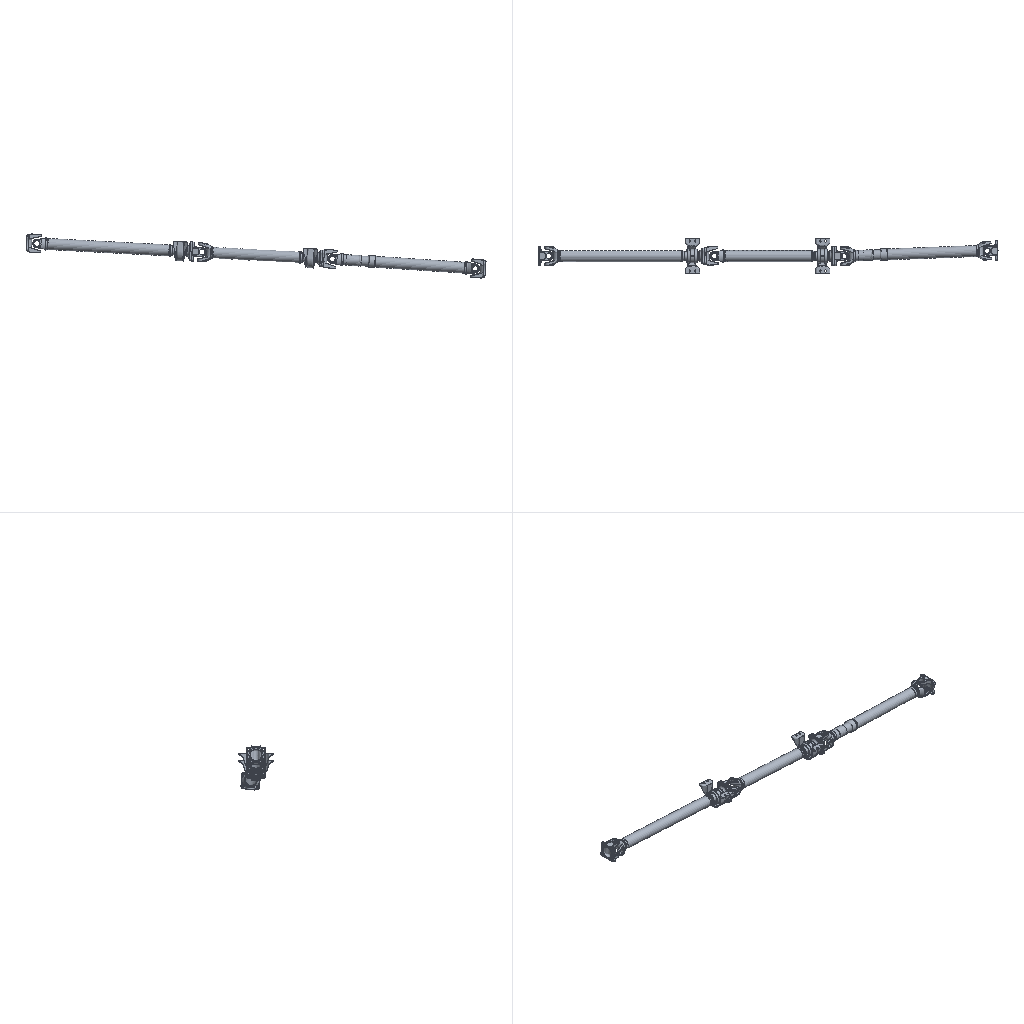Simulation study | nastran
Set-up summary:
category,name,step,type,value,unit,region
solver,nx_nastran
units,not stated in the deck,,not stated
analysis,deck,,modal,modal
analysis,solution,,SOL,103
load_step,SUBCASE 1,1,SUBCASE,SPC=1 LOAD=None
mesh,nodes,,,200329
mesh,elements,,,777144
element_type,CQUAD4,,shell,9182
element_type,CTETRA,,solid,767674
element_type,CTRIA3,,shell,288
load,load commands in deck,,count,0
bc,support commands in deck,,count,16
check,setup vs results,,match,"every grid point's frame and coordinates and every element id; grid points of CQUAD4, CTETRA, CTRIA3 elements"
Nastran input file, long lists of numbers shortened:
$$------------------------------------------------------------------------------$
$$                                                                              $
$$ NASTRAN Input Deck Generated by HyperMesh Version  :10.0buil                 $
$$ Generated using HyperMesh-Nastran Template Version : 10.0build60
$$                                                                              $
$$   Template:  general                                                         $
$$                                                                              $
$$------------------------------------------------------------------------------$
$$------------------------------------------------------------------------------$
$$                      Executive Control Cards                                 $
$$------------------------------------------------------------------------------$
SOL 103
CEND
$$------------------------------------------------------------------------------$
$$                      Case Control Cards                                      $
$$------------------------------------------------------------------------------$
  DISPLACEMENT = ALL
$
$HMNAME LOADSTEP               1"modal"
SUBCASE       1
  LABEL=  modal
  SPC =        1
  METHOD(STRUCTURE) =        2
$$------------------------------------------------------------------------------$
$$                      Bulk Data Cards                                         $
$$------------------------------------------------------------------------------$
BEGIN BULK
PARAM,POST,-1
$$
$$  GRID Data
$$
GRID           1        4926.96494.71653-393.548
GRID           2        4929.61194.74233-394.182
$ (200327 more lines like these left out)
$$
$$  SPOINT Data
$$
$$
$$------------------------------------------------------------------------------$
$$             Group Definitions                                                $
$$------------------------------------------------------------------------------$
$
$ RBE2 Elements - Single dependent node
$
RBE2      149214   28273   12346   28272
RBE2      618930  160318   12346  160317
$
$HMMOVE       10
$         149214  618930
$
$$
$$ RBE2 Elements - Multiple dependent nodes
$$
RBE2      149212   28272   12345    3911    3912    3913    3914    3915+
+           3916    3917    3918    3919    3920    3921    3922    4886+
+           4887    4888    4889    4890    4891    4892    4893    4894+
+           4895    4896    4897    4898    4899    4900    4901    4902+
+           4903    4904    4905    4906    4907    4908    4909    4910+
+           4911    4912    4913    4914    4915    4916    4917    4918+
+           4919    4920    4921    4922    4923    4924    4925    4926+
+           4927    4928    4929    4930    4931    4932    4933    4934+
+           5993    5994    5995    5996    5997    5998    5999    6000+
+           6001    6002    6003    6004    6005    6006    6007    6008+
+           6009    6010    6011    6012    6013    6014    6015    6016+
+           6017    6018    6179    6180    6181    6182    6183    6184+
+           6185    6186    6187    6188    6189    6190    6191    6192+
+           6193    6194    6195    6196    6197    6198    6199    6200+
+           6201    6202    6203    6204    6205    6206    6207    6208+
+           6209    6210    6211    6212    6213    6214    6215    6216+
+           6217    6218    6219    6220    6221    6222    6223    6224+
+           6225    6226    6227    6228    6229    6230    6231    6232+
+           6233    6234    6235    6236    6237    6238    6239    6240+
+           6241    6242    6243    6244    6245    6246    6247    6248+
+           6249    6250    6251    6252    6253    6254    6255    6256+
+           6257    6258    6259    6260    6261    6262    6263    6264+
+           6265    6266    6267    6268    6269    6270    6271    6272+
+           6273    6274    6275    6276    6277    6278    6279    6280+
+           6281    6282    6283    6284    6285    6286    6287    6288+
+           6289    6290    6291    6292    6293    6294    6295    6296+
+           6297    6298    6299    6300    6301    6302    6303    6304+
+           6305    6306    6307    6308    6309    6310    6311    6312+
+           6313    6314    6315    6316    6317    6318    6319    6320+
+           6321    6322    6323    6324    6325    6326    6327    6328+
+           6329    6330    6331    6332    6333    6334    6335    6336+
+           6337    6338    6339    6340    6341    6342    6343    6344+
+           6345    6346    6347    6348    6349    6350    6351    6352+
+           6353    6354    6355    6356    6357    6358    6359    6360+
+           6361    6362    6363    6364    6365    6366    6367    6368+
+           6369    6370    6371    6372    6373    6374    6375    6376+
+           6377    6378    6379    6380    6381    6382    6383    6384+
+           6385    6386    6387    6388    6389    6390    6391    6392+
+           6393    6394    6395    6396    6397    6398    6399    6400+
+           6401    6402    6403    6404    6405    6406    6407    6408+
+           6409    6410    6411    6412    6413    6414    6415    6416+
+           6417    6418    6419    6420    6421    6422    6423    6424+
+           6425    6426    6427    6428    6429    6430    6431    6432+
+           6433    6434    6435    6436    6437    6438    6439    6440+
+           6441    6442    6443    6444    6445    6446    6447    6448+
+           6449    6450    6451    6452    6453    6454    6455    6456+
+           6457    6458    6459    6460    6461    6462    6463    6464+
+           6465    6466    6467    6468    6469    6470    6471    6472+
+           6473    6474    6475    6476    6477    6478    6479    6480+
+           6481    6482    6483    6484    6485    6486    6487    6488+
+           6489    6490    6491    6492    6493    6494    6495    6496+
+           6497    6498    6499    6500    6501    6502    6503    6504+
+           6505    6506    6507    6508    6509    6510    6511    6512+
+           6513    6514    6515    6516    6517    6518    6519    6520+
+           6521    6522    6523    6524    6525    6526    6527    6528+
+           6529    6530    6531    6532    6533    6534    6535    6536+
+           6537    6538    6539    6540    6541    6542    6543    6544+
+           6545    6546    6547    6548    6549    6550    6551    6552+
+           6553    6554    6555    6556    6557    6558    6559    6560+
+           6561    6562    6563    6564    6565    6566    6567    6568+
+           6569    6570    6571    6572    6573    6574    6575    6576+
+           6577    6578    6579    6580    6581    6582    6583    6584+
+           6585    7297    7298    7299    7300    7301    7302    7303+
+           7304    7305    7306    7307    7308    7309    7310    7311+
+           7312    7313    7314    7315    7316    7317    7318    7319+
+           7320    7321    7322    7323    7324    7325    7326    7327+
+           7328    7329    7330    7331    7332    7333    7334    7335+
+           7336    7337    7338    7339    7340    7341    7342    7343+
+           7344    7345    8395    8396    8397    8398    8399    8400+
+           8401    8402    8403    8404    8405    8406    8407    8408+
+           8409    8410    8411    8412    8413    8414    8415    8416+
+           8417    8418    8419    8420    8421    8422    8423    8424+
+           8425    8426    8427    8428    8429    8430    8431    8432+
+           8433    8434    8435    8436    8437    8438    8439    8440+
+           8441    8442    8443    8444    8445    8446    8447    8448+
+           8449    8450    8451    8452    8453    8454    8455    8456+
+           8457    8458    8459    8460    8461    8462    8463    8464+
+           8465    8466    8467    8468    8469    8470    8471    8472+
+           8473    8474    8475    8476    8477    8478    8479    8480+
+           8481    8482    8483    8484    8485    8486    8487    8488+
+           8489    8490    8491    8492    8493    8494    8495    8496+
+           8497    8498    8499    8500    8501    8502    8503    8504+
+           8505    8506    8507    8508    8509    8510    8511    8512+
+           8513    8514    8515    8516    8517    8518    8519    8520+
+           8521    8522    8523    8524    8525    8526    8527    8528+
+           8529    8530    8531    8532    8533    8534    8535    8536+
+           8537    8538    8539    8540    8541    8542    8543    8544+
+           8545    8546    8547    8548    8549    8550    8551    8552+
+           8553    8554    8555    8556    8557    8558    8559    8560+
+           8561    8562    8563    8564    8565    8566    8567    8568+
+           8569    8570    8571    8572    8573    8574    8575    8576+
+           8577    8578    8579    8580    8581    8582    8583    8584+
+           8585    8586    8587    8588    8589    8590    8591    8592+
+           8593    8594    8595    8596    8597    8598    8599    8600+
+           8601    8602    8603    8604    8605    8606    8607    8608+
+           8609    8610    8611    8612    8613    8614    8615    8616+
+           8617    8618    8619    8620    8621    8622    8623    8624+
+           8625    8626    8627    8628    8629    8630    8631    8632+
+           8633    8634    8635    8636    8637    8638    8639    8640+
+           8641    8642    8643    8644    8645    8646    8647    8648+
+           8649    8650    8651    8652    8653    8654    8655    8656+
+           8657    8658    8659    8660    8661    8662    8663    8664+
+           8665    8666    8667    8668    8669    8670    8671    8672+
+           8673    8674    8675    8676    8677    8678    8679    8680+
+           8681    8682    8683    8684    8685    8686    8687    8688+
+           8689    8690    8691    8692    8693    8694    8695    8696+
+           8697    8698    8699    8700    8701    8702    8703    8704+
+           8705    8706    8707    8708    8709    8710    8711    8712+
+           8713    8714    8715    8716    8717    8718    8719    8720+
+           8721    8722    8723    8724    8725    8726    8727    8728+
+           8729    8730    8731    8732    8733    8734    8735    8736+
+           8737    8738    8739    8740    8741    8742    8743    8744+
+           8745    8746    8747    8748    8749    8750    8751    8752+
+           8753    8754    8755    8756    8757    8758    8759    8760+
+           8761    8762    8763    8764    8765    8766    8767    8768+
+           8769    8770    8771    8772    8773    8774    8775    8776+
+           8777    8778    8779    8780    8781    8782    8783    8784+
+           8785    8786    8787    8788    8789    8790    8791    8792+
+           8793    8794    8795    8796    8797    8798    8799    8800+
+           8801    8802    8803    8804    8805    8806    8807    8808+
+           8809    8810    8811    8812    8813    8814    8815    8816+
+           8817
RBE2      149213   28273   12346   15644   19611   19612   19613   19614+
+          19615   19616   19617   19618   19619   19620   19621   19622+
+          19623   19624   19625   19626   19627   19628   19629   19630+
+          19631   19632   19633   19634   19635   19636   19637   19948+
+          19949   20050   20051   20052   20053   20054   20055   20056+
+          20057   20058   20059   20060   20061   20062   20063   20064+
+          20065   20066   20067   20068   20069   20070   20071   20072+
+          20073   20074   20075   20076   20077   20078   20079   20080+
+          20081   20082   20083   20084   20085   20086   20087   20088+
+          20089   20090   20091   20092   20093   20094   20095   20096+
+          20097   20224   20422   20423   20424   20425   20426   20427+
+          20428   20429   20430   20431   20432   20433   20434   20435+
+          20436   20437   20438   20439   20440   20441   20442   20443+
+          20444   20445   20446   20447   20448   20449   20450   20451+
+          20452   20453   20454   20456   20457   20458   20459   20460+
+          20461   20462   20463   20464   20465   20466   20467   20468+
+          20469   20470   20471   20472   20473   20474   20475   20476+
+          20477   20478   20479   20480   20481   20482   20483   20484+
+          20485   20486   20487   20488   20489   20490   20491   20492+
+          20493   20494   20495   20496   20497   20498   20499   20500+
+          20501   20502   20503   20504   20505   20506   20507   20508+
+          20509   20510   20511   20512   20513   20514   20515   20516+
+          20517   20518   20519   20520   20521   20522   20523   20524+
+          20525   20526   20527   20528   20529   20530   20531   20532+
+          20533   20534   20535   20536   20537   20538   20539   20540+
+          20541   20542   20543   20544   20545   20546   20547   20548+
+          20549   20550   20551   20552   20553   20554   20555   20556+
+          20557   20558   20559   20560   20561   20562   20563   20564+
+          20565   20566   20567   20568   20569   20570   20571   20572+
+          20573   20574   20575   20576   20577   20578   20579   20580+
+          20581   20582   20583   20584   20585   20586   20587   20588+
+          20589   20590   20591   20592   20593   20594   20595   20596+
+          20597   20598   20599   20600   20601   20602   20603   20604+
+          20605   20606   20607   20608   20609   20610   20611   20612+
+          20613   20614   20615   20616   20617   20618   20619   20620+
+          20621   20622   20623   20624   20625   20626   20627   20628+
+          20629   20630   20631   20632   20633   20634   20635   20636+
+          20637   20638   20639   20640   20641   20642   20643   20644+
+          20645   20646   20647   20648   20649   20650   20651   20652+
+          20653   20654   20655   20656   20657   20658   20659   20660+
+          20661   20662   20663   20664   20665   20666   20667   20668+
+          20669   20670   20671   20672   20673   20674   20675   20676+
+          20677   20678   20679   20680   20681   20682   20683   20684+
+          20685   20686   20687   20688   20689   20690   20691   20692+
+          20693   20694   20695   20696   20697   20698   20699   20700+
+          20701   20702   20703   20704   20705   20706   20707   20708+
+          20709   20710   20711   20712   20713   20714   20715   20716+
+          20717   20718   20719   20720   20721   20722   20723   20724+
+          20725   20726   20727   20728   20729   20730   20731   20732+
+          20733   20734   20735   20736   20737   20738   20739   20740+
+          20741   20742   20743   20744   20745   20746   20747   20748+
+          20749   20750   20751   20752   20753   20754   20755   20756+
+          20757   20758   20759   20760   20761   20762   20763   20764+
+          20765   20766   20767   20768   20769   20770   20771   20772+
+          20773   20774   20775   20776   20777   20778   20779   20780+
+          20781   20782   20783   20784   20785   20786   20787   20788+
+          20789   20790   20791   20792   20793   20794   20795   20796+
+          20797   20798   20799   20800   20801   20802   20803   20804+
+          20805   20806   20807   20808   20809   20810   20811   20812+
+          20813   20814   20815   20816   20817   20818   20819   20820+
+          20821   20822   20823   20824   20825   20826   20827   20828+
+          20829   20849   20850   20921   21002   21011   21012   21013+
+          21014   21015   21016   21017   21018   21019   21020   21021+
+          21022   21023   21024   21025   21026   21027   21028   21029+
+          21030   21031   21032   21033   21034   21035   21036   21037+
+          21038   21039   21040   21041   21042   21043   21044   21045+
+          21046   21047   21048   21049   21050   21051   21052   21053+
+          21054   21055   21056   21057   21058   21059   21060   21061+
+          21062   21063   21064   21066   21067   21068   21069   21070+
+          21071   21072   21073   21074   21075   21076   21077   21078+
+          21079   21080   21081   21082   21083   21084   21085   21086+
+          21087   21088   21089   21090   21091   21092   21093   21094+
+          21095   21096   21097   21098   21099   21100   21101   21102+
+          21103   21104   21105   21106   21107   21108   21109   21110+
+          21111   21112   21113   21114   21115   21116   21117   21118+
+          21119   21120   21121   21122   21123   21124   21125   21126+
+          21127   21128   21129   21130   21131   21132   21133   21134+
+          21135   21136   21137   21138   21139   21140   21141   21142+
+          21143   21144   21145   21146   21147   21148   21149   21150+
+          21151   21152   21153   21154   21155   21156   21157   21158+
+          21159   21160   21161   21162   21163   21164   21165   21166+
+          21167   21168   21169   21170   21171   21172   21173   21174+
+          21175   21176   21177   21178   21179   21180   21181   21182+
+          21183   21184   21185   21186   21187   21188   21189   21190+
+          21191   21192   21193   21194   21195   21196   21197   21198+
+          21199   21200   21201   21202   21203   21204   21205   21206+
+          21207   21208   21209   21210   21211   21212   21213   21214+
+          21215   21216   21217   21218   21219   21220   21221   21222+
+          21223   21224   21225   21226   21227   21228   21229   21230+
+          21231   21232   21233   21234   21235   21236   21237   21238+
+          21239   21240   21241   21242   21243   21244   21245   21246+
+          21247   21248   21249   21250   21251   21252   21253   21254+
+          21255   21256   21257   21258   21259   21260   21261   21262+
+          21263   21264   21265   21266   21267   21268   21269   21270+
+          21271   21272   21347   21348   21349   21350   21351   21352+
+          21353   21354   21355   21356   21357   21358   21359   21360+
+          21361   21362   21363   21364   21365   21366   21367   21368+
+          21369   21370   21371   21522   21523   21524   21525   21526+
+          21527   21528   21529   21530   21531   21532   21533   21534+
+          21535   21536   21537   21538   21539   21540   21541   21542+
+          21543   21544   21545   21546   21547   21548   21549   21550+
+          21551   21552   21553   21554   21555   21556   21557   21558+
+          21559   21560   21561   21562   21563   21564   21565   21566+
+          21567   21568   21569   21570   21571   21572   21573   21574+
+          21575   21576   21577   21578   21579   21580   21581   21582+
+          21583   21584   21585   21586   21587   21588   21589   21590+
+          21591   21592   21593   21594   21595   21596   21597   21598+
+          21599   21600   21601   21602   21603   21604   21605   21606+
+          21607   21608   21609   21610   21611   21612   21613   21614+
+          21615   21616   21617   21618   21619   21620   21621   21622+
+          21623   21624   21625   21626   21627   21628   21629   21630+
+          21631   21632   21633   21634   21635   21636   21637   21638+
+          21639   21640   21641   21642   21643   21644   21645   21646+
+          21647   21648   21649   21650   21651   21652   21653   21654+
+          21655   21656   21657   21658   21659   21660   21661   21662+
+          21663   21664   21665   21666   21667   21668   21669   21670+
+          21671   21672   21673   21674   21675   21676   21677   21678+
+          21679   21680   21681   21682   21683   21684   21685   21686+
+          21687   21688   21689   21690   21691   21692   21693   21694+
+          21695   21696   21697   21698   21699   21700   21701   21702+
+          21703   21704   21705   21706   21707   21708   21709   21710+
+          21711   21712   21713   21714   21715   21716   23572   23581+
+          23903   23923   24056   24112   24149   24175   24338   24991+
+          25053   25661   25754   25850   25882   26058   26122   26206+
+          26284   27081
$ (4446 more lines like these left out)
$
$HMMOVE       10
$         149212THRU      149213  618928THRU      618929 1615586 2102630THRU
$        2102634 2707187THRU     2707188 2720047 2756158 2808651THRU     2808655
$        2821514 2857625 2883872THRU     2883876 2921815THRU     2921817 2937534
$        2965317THRU     2965330 2965332THRU     2965335
$
$$
$$  CTRIA3 Data
$$
CTRIA3    487045       2   91878   91865   91864
CTRIA3    487058       2   91889   91841   91840
$ (286 more lines like these left out)
$
$HMMOVE       18
$         487045  487058
$
$ (44 more lines like these left out)
CQUAD4    484907       2   89874   89876   89871   89872
CQUAD4    484908       2   89876   89867   89868   89871
$ (9180 more lines like these left out)
$
$HMMOVE       11
$         484907THRU      486674
$
$ (131 more lines like these left out)
CTETRA     57097       1   13870   13402   11223   13788
CTETRA     57098       1   14799   14445   10888   11624
$ (767672 more lines like these left out)
$
$HMMOVE        6
$          57097THRU       58096   38968THRU       38972   56102THRU       57096
$          38923THRU       38967   55147THRU       56101   38915THRU       38922
$ (250 more lines like these left out)
PSHELL         2       15.0            1               1
$$
$$  PSOLID Data
$
$HMNAME PROP                   1"psolid" 5
$HWCOLOR PROP                  1       4
PSOLID         1       1
$$
$$------------------------------------------------------------------------------$
$$                      Material Definition Cards                               $
$$------------------------------------------------------------------------------$
$$--------------------------------------------------------------
$$ HYPERMESH TAGS
$$--------------------------------------------------------------
$$BEGIN TAGS
$$END TAGS
$$
$$  MAT1 Data
$
$HMNAME MAT                    1"steel" "MAT1"
$HWCOLOR MAT                   1       3
MAT1           1210000.0        0.3     7.90E-09
$$
$$
$$
$$------------------------------------------------------------------------------$
$ (34 more lines like these left out)
EIGRL          20.0                   10                            MASS
$$
$$  SPC Data
$$
SPC            1  366060  1234560.0
SPC            1  366061  1234560.0
SPC            1  366062  1234560.0
SPC            1  366063  1234560.0
SPC            1  366064  1234560.0
SPC            1  366065  1234560.0
SPC            1  366066  1234560.0
SPC            1  366067  1234560.0
SPC            1  366068  1234560.0
SPC            1  366069  1234560.0
SPC            1  366070  1234560.0
SPC            1  366071  1234560.0
SPC            1  366073  1234560.0
SPC            1  366074  1234560.0
SPC            1  366075  1234560.0
SPC            1  366076  1234560.0
$HMASSEM       1       3 2200011G1060
$HMASSEM_ASSEM_ID              2
$HMASSEM       2       4 2200011G1060.2
$HMASSEM       3       5 2200030G1810
$HMASSEM_ASSEM_ID              4
$HMASSEM       4       6 2200030G1810.3
$HMASSEM       5       7 2201100LG010
$HMASSEM_ASSEM_ID              6
$HMASSEM       6       8 2201100LG010.4
$HMASSEM       7       9 2202100LG010
$HMASSEM_ASSEM_ID              8
$HMASSEM       8      13 2202100LG010.5
$HMASSEM       9      17 2204100LG010
$HMASSEM_ASSEM_ID             10
$HMASSEM      10      20 2204100LG010.6
$HMASSEM      11       5 2200
$HMASSEM_IDS           6       7      10      11      13      18      19      20
$HMASSEM_IDS          21      22      30      31      35      36      37      38
$HMASSEM_IDS          39      41      42      43
$
ENDDATA
Results summary:
result,analysis,,,modal
result,primary field,,,eigenvectors